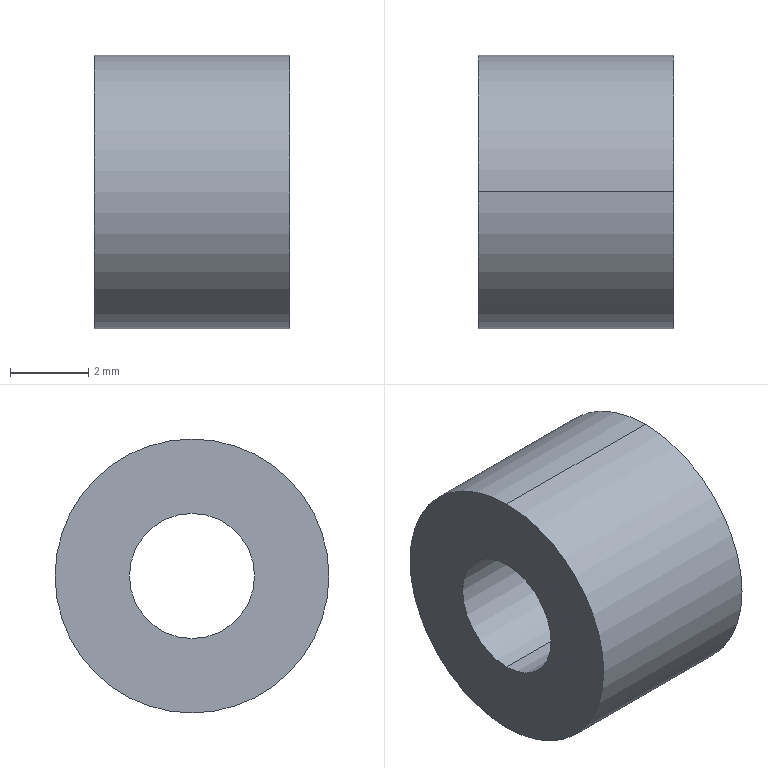Part | SolidWorks | features Extrusion 1 | 1 solid | 6 faces | box 5 x 7 x 7 mm | volume 152.21 mm3 | cylinder 4 | plane 2 | commonest cylinder face diameters 3.2 x2 7 x2
STEP:
#1=CARTESIAN_POINT('',(5.,0.,1.6));
#2=VERTEX_POINT('',#1);
#3=CARTESIAN_POINT('',(5.,0.,-1.6));
#4=VERTEX_POINT('',#3);
#5=CARTESIAN_POINT('',(5.,0.,0.));
#6=DIRECTION('',(1.,0.,0.));
#7=DIRECTION('',(0.,0.,-1.));
#8=AXIS2_PLACEMENT_3D('',#5,#6,#7);
#9=CIRCLE('',#8,1.6);
#10=EDGE_CURVE('',#2,#4,#9,.T.);
#11=ORIENTED_EDGE('',*,*,#10,.T.);
#12=CARTESIAN_POINT('',(0.,0.,-1.6));
#13=VERTEX_POINT('',#12);
#14=CARTESIAN_POINT('',(5.,0.,-1.6));
#15=DIRECTION('',(-1.,0.,0.));
#16=VECTOR('',#15,1000.);
#17=LINE('',#14,#16);
#18=EDGE_CURVE('',#4,#13,#17,.T.);
#19=ORIENTED_EDGE('',*,*,#18,.T.);
#20=CARTESIAN_POINT('',(0.,0.,1.6));
#21=VERTEX_POINT('',#20);
#22=CARTESIAN_POINT('',(0.,0.,0.));
#23=DIRECTION('',(1.,0.,0.));
#24=DIRECTION('',(0.,0.,-1.));
#25=AXIS2_PLACEMENT_3D('',#22,#23,#24);
#26=CIRCLE('',#25,1.6);
#27=EDGE_CURVE('',#21,#13,#26,.T.);
#28=ORIENTED_EDGE('',*,*,#27,.F.);
#29=CARTESIAN_POINT('',(5.,0.,1.6));
#30=DIRECTION('',(-1.,0.,0.));
#31=VECTOR('',#30,1000.);
#32=LINE('',#29,#31);
#33=EDGE_CURVE('',#2,#21,#32,.T.);
#34=ORIENTED_EDGE('',*,*,#33,.F.);
#35=EDGE_LOOP('',(#11,#19,#28,#34));
#36=FACE_OUTER_BOUND('',#35,.T.);
#37=CARTESIAN_POINT('',(5.,0.,0.));
#38=DIRECTION('',(-1.,0.,0.));
#39=DIRECTION('',(0.,0.,1.));
#40=AXIS2_PLACEMENT_3D('',#37,#38,#39);
#41=CYLINDRICAL_SURFACE('',#40,1.6);
#42=ADVANCED_FACE('',(#36),#41,.F.);
#43=CARTESIAN_POINT('',(5.,0.,-3.5));
#44=VERTEX_POINT('',#43);
#45=CARTESIAN_POINT('',(5.,0.,3.5));
#46=VERTEX_POINT('',#45);
#47=CARTESIAN_POINT('',(5.,0.,0.));
#48=DIRECTION('',(1.,0.,0.));
#49=DIRECTION('',(0.,0.,-1.));
#50=AXIS2_PLACEMENT_3D('',#47,#48,#49);
#51=CIRCLE('',#50,3.5);
#52=EDGE_CURVE('',#44,#46,#51,.T.);
#53=ORIENTED_EDGE('',*,*,#52,.F.);
#54=CARTESIAN_POINT('',(0.,0.,-3.5));
#55=VERTEX_POINT('',#54);
#56=CARTESIAN_POINT('',(5.,0.,-3.5));
#57=DIRECTION('',(-1.,0.,0.));
#58=VECTOR('',#57,1000.);
#59=LINE('',#56,#58);
#60=EDGE_CURVE('',#44,#55,#59,.T.);
#61=ORIENTED_EDGE('',*,*,#60,.T.);
#62=CARTESIAN_POINT('',(0.,0.,3.5));
#63=VERTEX_POINT('',#62);
#64=CARTESIAN_POINT('',(0.,0.,0.));
#65=DIRECTION('',(1.,0.,0.));
#66=DIRECTION('',(0.,0.,-1.));
#67=AXIS2_PLACEMENT_3D('',#64,#65,#66);
#68=CIRCLE('',#67,3.5);
#69=EDGE_CURVE('',#55,#63,#68,.T.);
#70=ORIENTED_EDGE('',*,*,#69,.T.);
#71=CARTESIAN_POINT('',(5.,0.,3.5));
#72=DIRECTION('',(-1.,0.,0.));
#73=VECTOR('',#72,1000.);
#74=LINE('',#71,#73);
#75=EDGE_CURVE('',#46,#63,#74,.T.);
#76=ORIENTED_EDGE('',*,*,#75,.F.);
#77=EDGE_LOOP('',(#53,#61,#70,#76));
#78=FACE_OUTER_BOUND('',#77,.T.);
#79=CARTESIAN_POINT('',(5.,0.,0.));
#80=DIRECTION('',(-1.,0.,0.));
#81=DIRECTION('',(0.,0.,1.));
#82=AXIS2_PLACEMENT_3D('',#79,#80,#81);
#83=CYLINDRICAL_SURFACE('',#82,3.5);
#84=ADVANCED_FACE('',(#78),#83,.T.);
#85=CARTESIAN_POINT('',(5.,0.,0.));
#86=DIRECTION('',(1.,0.,0.));
#87=DIRECTION('',(0.,0.,-1.));
#88=AXIS2_PLACEMENT_3D('',#85,#86,#87);
#89=CIRCLE('',#88,3.5);
#90=EDGE_CURVE('',#46,#44,#89,.T.);
#91=ORIENTED_EDGE('',*,*,#90,.T.);
#92=ORIENTED_EDGE('',*,*,#52,.T.);
#93=EDGE_LOOP('',(#91,#92));
#94=FACE_OUTER_BOUND('',#93,.T.);
#95=ORIENTED_EDGE('',*,*,#10,.F.);
#96=CARTESIAN_POINT('',(5.,0.,0.));
#97=DIRECTION('',(1.,0.,0.));
#98=DIRECTION('',(0.,0.,-1.));
#99=AXIS2_PLACEMENT_3D('',#96,#97,#98);
#100=CIRCLE('',#99,1.6);
#101=EDGE_CURVE('',#4,#2,#100,.T.);
#102=ORIENTED_EDGE('',*,*,#101,.F.);
#103=EDGE_LOOP('',(#95,#102));
#104=FACE_BOUND('',#103,.T.);
#105=CARTESIAN_POINT('',(5.,0.,0.));
#106=DIRECTION('',(1.,0.,0.));
#107=DIRECTION('',(0.,0.,-1.));
#108=AXIS2_PLACEMENT_3D('',#105,#106,#107);
#109=PLANE('',#108);
#110=ADVANCED_FACE('',(#94,#104),#109,.T.);
#111=CARTESIAN_POINT('',(0.,0.,0.));
#112=DIRECTION('',(1.,0.,0.));
#113=DIRECTION('',(0.,0.,-1.));
#114=AXIS2_PLACEMENT_3D('',#111,#112,#113);
#115=CIRCLE('',#114,3.5);
#116=EDGE_CURVE('',#63,#55,#115,.T.);
#117=ORIENTED_EDGE('',*,*,#116,.F.);
#118=ORIENTED_EDGE('',*,*,#69,.F.);
#119=EDGE_LOOP('',(#117,#118));
#120=FACE_OUTER_BOUND('',#119,.T.);
#121=ORIENTED_EDGE('',*,*,#27,.T.);
#122=CARTESIAN_POINT('',(0.,0.,0.));
#123=DIRECTION('',(1.,0.,0.));
#124=DIRECTION('',(0.,0.,-1.));
#125=AXIS2_PLACEMENT_3D('',#122,#123,#124);
#126=CIRCLE('',#125,1.6);
#127=EDGE_CURVE('',#13,#21,#126,.T.);
#128=ORIENTED_EDGE('',*,*,#127,.T.);
#129=EDGE_LOOP('',(#121,#128));
#130=FACE_BOUND('',#129,.T.);
#131=CARTESIAN_POINT('',(0.,0.,0.));
#132=DIRECTION('',(1.,0.,0.));
#133=DIRECTION('',(0.,0.,-1.));
#134=AXIS2_PLACEMENT_3D('',#131,#132,#133);
#135=PLANE('',#134);
#136=ADVANCED_FACE('',(#120,#130),#135,.F.);
#137=ORIENTED_EDGE('',*,*,#60,.F.);
#138=ORIENTED_EDGE('',*,*,#90,.F.);
#139=ORIENTED_EDGE('',*,*,#75,.T.);
#140=ORIENTED_EDGE('',*,*,#116,.T.);
#141=EDGE_LOOP('',(#137,#138,#139,#140));
#142=FACE_OUTER_BOUND('',#141,.T.);
#143=CARTESIAN_POINT('',(5.,0.,0.));
#144=DIRECTION('',(-1.,0.,0.));
#145=DIRECTION('',(0.,0.,1.));
#146=AXIS2_PLACEMENT_3D('',#143,#144,#145);
#147=CYLINDRICAL_SURFACE('',#146,3.5);
#148=ADVANCED_FACE('',(#142),#147,.T.);
#149=ORIENTED_EDGE('',*,*,#18,.F.);
#150=ORIENTED_EDGE('',*,*,#101,.T.);
#151=ORIENTED_EDGE('',*,*,#33,.T.);
#152=ORIENTED_EDGE('',*,*,#127,.F.);
#153=EDGE_LOOP('',(#149,#150,#151,#152));
#154=FACE_OUTER_BOUND('',#153,.T.);
#155=CARTESIAN_POINT('',(5.,0.,0.));
#156=DIRECTION('',(-1.,0.,0.));
#157=DIRECTION('',(0.,0.,1.));
#158=AXIS2_PLACEMENT_3D('',#155,#156,#157);
#159=CYLINDRICAL_SURFACE('',#158,1.6);
#160=ADVANCED_FACE('',(#154),#159,.F.);
#161=CLOSED_SHELL('',(#42,#84,#110,#136,#148,#160));
#162=MANIFOLD_SOLID_BREP('',#161);
#163=CARTESIAN_POINT('',(0.,0.,0.));
#164=DIRECTION('',(0.,0.,1.));
#165=DIRECTION('',(1.,0.,0.));
#166=AXIS2_PLACEMENT_3D('',#163,#164,#165);
#167=(LENGTH_UNIT()NAMED_UNIT(*)SI_UNIT(.MILLI.,.METRE.));
#168=UNCERTAINTY_MEASURE_WITH_UNIT(LENGTH_MEASURE(0.00001),#167,'','');
#169=(NAMED_UNIT(*)PLANE_ANGLE_UNIT()SI_UNIT($,.RADIAN.));
#170=(NAMED_UNIT(*)SI_UNIT($,.STERADIAN.)SOLID_ANGLE_UNIT());
#171=(GEOMETRIC_REPRESENTATION_CONTEXT(3)GLOBAL_UNCERTAINTY_ASSIGNED_CONTEXT((#168))GLOBAL_UNIT_ASSIGNED_CONTEXT((#167,#169,#170))REPRESENTATION_CONTEXT('',''));
#172=ADVANCED_BREP_SHAPE_REPRESENTATION('',(#162,#166),#171);